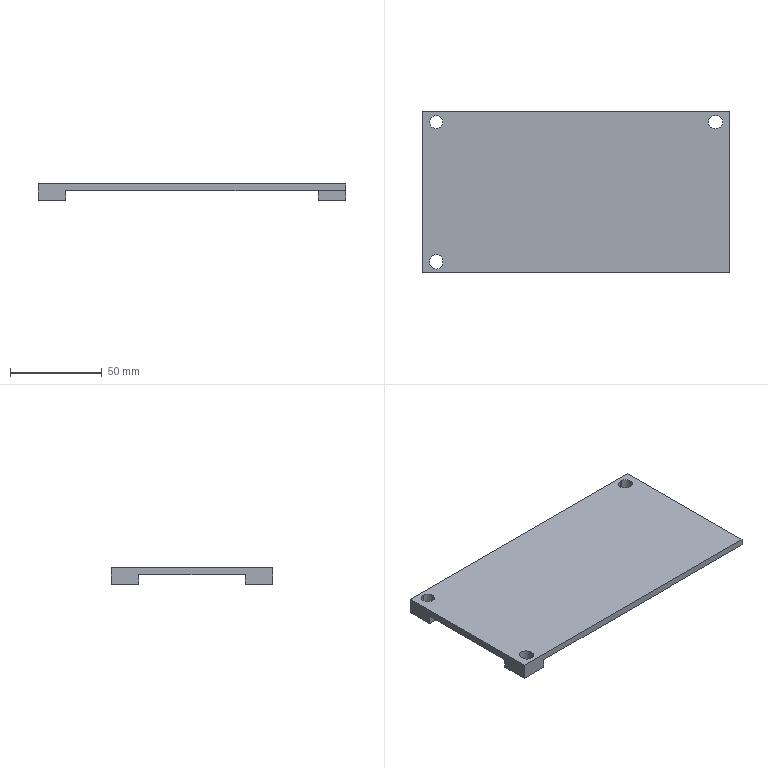NC program | NX | posted with a generic post | part box 168 x 88.2 x 8.8 mm
Lines 883 to 1702 of 6992:
(ZLEVEL_PROFILE , TOOL : D4)
N1752 T11 M6
N1754 G54
N1756 G17 G0 G90 X77.772 Y39.189 S9500 M3
N1758 G43 Z30. H11
N1760 Z1.5
N1762 G94 G1 X77.523 Y39.412 Z1.483 F1000.
N1764 X77.175 Y39.593 Z1.462
N1766 X76.793 Y39.685 Z1.441
N1768 X75.607 Z1.379
N1770 X75.225 Y39.594 Z1.359
N1772 X74.878 Y39.412 Z1.338
N1774 X74.585 Y39.151 Z1.318
N1776 X74.365 Y38.826 Z1.297
N1778 X74.239 Y38.492 Z1.278
N1780 X74.191 Y38.043 Z1.255
N1782 X74.271 Y37.597 Z1.231
N1784 X74.473 Y37.193 Z1.207
N1786 X74.781 Y36.861 Z1.183
N1788 X75.169 Y36.629 Z1.16
N1790 X75.607 Y36.515 Z1.136
N1792 X76.793 Z1.074
N1794 X77.231 Y36.629 Z1.05
N1796 X77.619 Y36.861 Z1.026
N1798 X77.927 Y37.192 Z1.003
N1800 X78.129 Y37.597 Z0.979
N1802 X78.209 Y38.042 Z0.955
N1804 X78.161 Y38.492 Z0.932
N1806 X78.036 Y38.825 Z0.913
N1808 X77.815 Y39.15 Z0.892
N1810 X77.523 Y39.412 Z0.872
N1812 X77.175 Y39.593 Z0.851
N1814 X76.793 Y39.685 Z0.831
N1816 X75.607 Z0.769
N1818 X75.225 Y39.594 Z0.748
N1820 X74.878 Y39.412 Z0.727
N1822 X74.585 Y39.151 Z0.707
N1824 X74.365 Y38.826 Z0.686
N1826 X74.239 Y38.492 Z0.668
N1828 X74.191 Y38.043 Z0.644
N1830 X74.271 Y37.597 Z0.62
N1832 X74.473 Y37.193 Z0.596
N1834 X74.781 Y36.861 Z0.573
N1836 X75.169 Y36.629 Z0.549
N1838 X75.607 Y36.515 Z0.525
N1840 X76.793 Z0.463
N1842 X77.231 Y36.629 Z0.439
N1844 X77.619 Y36.861 Z0.416
N1846 X77.927 Y37.192 Z0.392
N1848 X78.129 Y37.597 Z0.368
N1850 X78.209 Y38.042 Z0.345
N1852 X78.161 Y38.492 Z0.321
N1854 X78.036 Y38.825 Z0.302
N1856 X77.815 Y39.15 Z0.282
N1858 X77.523 Y39.412 Z0.261
N1860 X77.175 Y39.593 Z0.241
N1862 X76.793 Y39.685 Z0.22
N1864 X75.607 Z0.158
N1866 X75.225 Y39.594 Z0.137
N1868 X74.878 Y39.412 Z0.117
N1870 X74.585 Y39.151 Z0.096
N1872 X74.365 Y38.826 Z0.076
N1874 X74.239 Y38.492 Z0.057
N1876 X74.191 Y38.043 Z0.033
N1878 X74.271 Y37.597 Z0.01
N1880 X74.473 Y37.193 Z-0.014
N1882 X74.781 Y36.861 Z-0.038
N1884 X75.169 Y36.629 Z-0.062
N1886 X75.607 Y36.515 Z-0.085
N1888 X76.793 Z-0.148
N1890 X77.231 Y36.629 Z-0.171
N1892 X77.619 Y36.861 Z-0.195
N1894 X77.927 Y37.192 Z-0.219
N1896 X78.129 Y37.597 Z-0.242
N1898 X78.209 Y38.042 Z-0.266
N1900 X78.161 Y38.492 Z-0.29
N1902 X78.036 Y38.825 Z-0.308
N1904 X77.815 Y39.15 Z-0.329
N1906 X77.523 Y39.412 Z-0.35
N1908 X77.175 Y39.593 Z-0.37
N1910 X76.793 Y39.685 Z-0.391
N1912 X76.615 Z-0.4
N1914 X75.785 F2000.
N1916 G3 X74.2 Y38.1 R1.585
N1918 X75.785 Y36.515 R1.585
N1920 G1 X76.615
N1922 G3 X78.2 Y38.1 R1.585
N1924 X76.615 Y39.685 R1.585
N1926 G1 X75.785 Z-0.429
N1928 X75.625 Y39.677 Z-0.434
N1930 X75.467 Y39.653 Z-0.44
N1932 X75.349 Y39.624 Z-0.444
N1934 X75.248 Y39.591 Z-0.447
N1936 X75.163 Y39.558 Z-0.451
N1938 X75.046 Y39.502 Z-0.455
N1940 X74.953 Y39.449 Z-0.459
N1942 X74.883 Y39.404 Z-0.462
N1944 X74.779 Y39.325 Z-0.466
N1946 X74.699 Y39.255 Z-0.47
N1948 X74.64 Y39.196 Z-0.473
N1950 X74.554 Y39.098 Z-0.477
N1952 X74.49 Y39.014 Z-0.481
N1954 X74.444 Y38.945 Z-0.484
N1956 X74.378 Y38.83 Z-0.488
N1958 X74.332 Y38.734 Z-0.492
N1960 X74.302 Y38.659 Z-0.495
N1962 X74.258 Y38.526 Z-0.499
N1964 X74.232 Y38.416 Z-0.503
N1966 X74.217 Y38.33 Z-0.506
N1968 X74.203 Y38.192 Z-0.511
N1970 X74.2 Y38.079 Z-0.515
N1972 X74.204 Y37.991 Z-0.518
N1974 X74.219 Y37.853 Z-0.523
N1976 X74.241 Y37.742 Z-0.527
N1978 X74.263 Y37.657 Z-0.53
N1980 X74.308 Y37.525 Z-0.535
N1982 X74.353 Y37.421 Z-0.538
N1984 X74.392 Y37.343 Z-0.541
N1986 X74.464 Y37.224 Z-0.546
N1988 X74.53 Y37.132 Z-0.55
N1990 X74.586 Y37.064 Z-0.553
N1992 X74.681 Y36.963 Z-0.558
N1994 X74.765 Y36.887 Z-0.562
N1996 X74.834 Y36.832 Z-0.565
N1998 X74.949 Y36.754 Z-0.57
N2000 X75.047 Y36.697 Z-0.574
N2002 X75.125 Y36.659 Z-0.577
N2004 X75.254 Y36.606 Z-0.581
N2006 X75.362 Y36.572 Z-0.585
N2008 X75.447 Y36.551 Z-0.588
N2010 X75.615 Y36.524 Z-0.594
N2012 X75.785 Y36.515 Z-0.6
N2014 X76.615 Z-0.629
N2016 X76.766 Y36.522 Z-0.634
N2018 X76.878 Y36.537 Z-0.638
N2020 X76.952 Y36.551 Z-0.64
N2022 X77.088 Y36.587 Z-0.645
N2024 X77.195 Y36.625 Z-0.649
N2026 X77.274 Y36.659 Z-0.652
N2028 X77.398 Y36.722 Z-0.657
N2030 X77.495 Y36.782 Z-0.661
N2032 X77.566 Y36.832 Z-0.664
N2034 X77.674 Y36.92 Z-0.669
N2036 X77.755 Y36.999 Z-0.672
N2038 X77.814 Y37.064 Z-0.675
N2040 X77.901 Y37.173 Z-0.68
N2042 X77.963 Y37.267 Z-0.684
N2044 X78.007 Y37.343 Z-0.687
N2046 X78.068 Y37.468 Z-0.692
N2048 X78.11 Y37.573 Z-0.696
N2050 X78.137 Y37.657 Z-0.699
N2052 X78.17 Y37.792 Z-0.704
N2054 X78.188 Y37.903 Z-0.708
N2056 X78.196 Y37.991 Z-0.711
N2058 X78.2 Y38.13 Z-0.715
N2060 X78.194 Y38.243 Z-0.719
N2062 X78.183 Y38.33 Z-0.722
N2064 X78.157 Y38.465 Z-0.727
N2066 X78.127 Y38.574 Z-0.731
N2068 X78.098 Y38.658 Z-0.734
N2070 X78.048 Y38.778 Z-0.738
N2072 X77.999 Y38.873 Z-0.742
N2074 X77.956 Y38.944 Z-0.745
N2076 X77.882 Y39.052 Z-0.749
N2078 X77.815 Y39.135 Z-0.753
N2080 X77.76 Y39.196 Z-0.756
N2082 X77.666 Y39.287 Z-0.76
N2084 X77.584 Y39.355 Z-0.764
N2086 X77.517 Y39.403 Z-0.767
N2088 X77.406 Y39.473 Z-0.771
N2090 X77.312 Y39.523 Z-0.775
N2092 X77.237 Y39.558 Z-0.778
N2094 X77.115 Y39.604 Z-0.782
N2096 X77.013 Y39.634 Z-0.786
N2098 X76.933 Y39.653 Z-0.789
N2100 X76.775 Y39.677 Z-0.794
N2102 X76.615 Y39.685 Z-0.8
N2104 X75.785 Z-0.829
N2106 X75.625 Y39.677 Z-0.834
N2108 X75.467 Y39.653 Z-0.84
N2110 X75.349 Y39.624 Z-0.844
N2112 X75.248 Y39.591 Z-0.847
N2114 X75.163 Y39.558 Z-0.851
N2116 X75.046 Y39.502 Z-0.855
N2118 X74.953 Y39.449 Z-0.859
N2120 X74.883 Y39.404 Z-0.862
N2122 X74.779 Y39.325 Z-0.866
N2124 X74.699 Y39.255 Z-0.87
N2126 X74.64 Y39.196 Z-0.873
N2128 X74.554 Y39.098 Z-0.877
N2130 X74.49 Y39.014 Z-0.881
N2132 X74.444 Y38.945 Z-0.884
N2134 X74.378 Y38.83 Z-0.888
N2136 X74.332 Y38.734 Z-0.892
N2138 X74.302 Y38.659 Z-0.895
N2140 X74.258 Y38.526 Z-0.899
N2142 X74.232 Y38.416 Z-0.903
N2144 X74.217 Y38.33 Z-0.906
N2146 X74.203 Y38.192 Z-0.911
N2148 X74.2 Y38.079 Z-0.915
N2150 X74.204 Y37.991 Z-0.918
N2152 X74.219 Y37.853 Z-0.923
N2154 X74.241 Y37.742 Z-0.927
N2156 X74.263 Y37.657 Z-0.93
N2158 X74.308 Y37.525 Z-0.935
N2160 X74.353 Y37.421 Z-0.938
N2162 X74.392 Y37.343 Z-0.941
N2164 X74.464 Y37.224 Z-0.946
N2166 X74.53 Y37.132 Z-0.95
N2168 X74.586 Y37.064 Z-0.953
N2170 X74.681 Y36.963 Z-0.958
N2172 X74.765 Y36.887 Z-0.962
N2174 X74.834 Y36.832 Z-0.965
N2176 X74.949 Y36.754 Z-0.97
N2178 X75.047 Y36.697 Z-0.974
N2180 X75.125 Y36.659 Z-0.977
N2182 X75.254 Y36.606 Z-0.981
N2184 X75.362 Y36.572 Z-0.985
N2186 X75.447 Y36.551 Z-0.988
N2188 X75.615 Y36.524 Z-0.994
N2190 X75.785 Y36.515 Z-1.
N2192 X76.615 Z-1.029
N2194 X76.766 Y36.522 Z-1.034
N2196 X76.878 Y36.537 Z-1.038
N2198 X76.952 Y36.551 Z-1.04
N2200 X77.088 Y36.587 Z-1.045
N2202 X77.195 Y36.625 Z-1.049
N2204 X77.274 Y36.659 Z-1.052
N2206 X77.398 Y36.722 Z-1.057
N2208 X77.495 Y36.782 Z-1.061
N2210 X77.566 Y36.832 Z-1.064
N2212 X77.674 Y36.92 Z-1.069
N2214 X77.755 Y36.999 Z-1.072
N2216 X77.814 Y37.064 Z-1.075
N2218 X77.901 Y37.173 Z-1.08
N2220 X77.963 Y37.267 Z-1.084
N2222 X78.007 Y37.343 Z-1.087
N2224 X78.068 Y37.468 Z-1.092
N2226 X78.11 Y37.573 Z-1.096
N2228 X78.137 Y37.657 Z-1.099
N2230 X78.17 Y37.792 Z-1.104
N2232 X78.188 Y37.903 Z-1.108
N2234 X78.196 Y37.991 Z-1.111
N2236 X78.2 Y38.13 Z-1.115
N2238 X78.194 Y38.243 Z-1.119
N2240 X78.183 Y38.33 Z-1.122
N2242 X78.157 Y38.465 Z-1.127
N2244 X78.127 Y38.574 Z-1.131
N2246 X78.098 Y38.658 Z-1.134
N2248 X78.048 Y38.778 Z-1.138
N2250 X77.999 Y38.873 Z-1.142
N2252 X77.956 Y38.944 Z-1.145
N2254 X77.882 Y39.052 Z-1.149
N2256 X77.815 Y39.135 Z-1.153
N2258 X77.76 Y39.196 Z-1.156
N2260 X77.666 Y39.287 Z-1.16
N2262 X77.584 Y39.355 Z-1.164
N2264 X77.517 Y39.403 Z-1.167
N2266 X77.406 Y39.473 Z-1.171
N2268 X77.312 Y39.523 Z-1.175
N2270 X77.237 Y39.558 Z-1.178
N2272 X77.115 Y39.604 Z-1.182
N2274 X77.013 Y39.634 Z-1.186
N2276 X76.933 Y39.653 Z-1.189
N2278 X76.775 Y39.677 Z-1.194
N2280 X76.615 Y39.685 Z-1.2
N2282 X75.785 Z-1.229
N2284 X75.625 Y39.677 Z-1.234
N2286 X75.467 Y39.653 Z-1.24
N2288 X75.349 Y39.624 Z-1.244
N2290 X75.248 Y39.591 Z-1.247
N2292 X75.163 Y39.558 Z-1.251
N2294 X75.046 Y39.502 Z-1.255
N2296 X74.953 Y39.449 Z-1.259
N2298 X74.883 Y39.404 Z-1.262
N2300 X74.779 Y39.325 Z-1.266
N2302 X74.699 Y39.255 Z-1.27
N2304 X74.64 Y39.196 Z-1.273
N2306 X74.554 Y39.098 Z-1.277
N2308 X74.49 Y39.014 Z-1.281
N2310 X74.444 Y38.945 Z-1.284
N2312 X74.378 Y38.83 Z-1.288
N2314 X74.332 Y38.734 Z-1.292
N2316 X74.302 Y38.659 Z-1.295
N2318 X74.258 Y38.526 Z-1.299
N2320 X74.232 Y38.416 Z-1.303
N2322 X74.217 Y38.33 Z-1.306
N2324 X74.203 Y38.192 Z-1.311
N2326 X74.2 Y38.079 Z-1.315
N2328 X74.204 Y37.991 Z-1.318
N2330 X74.219 Y37.853 Z-1.323
N2332 X74.241 Y37.742 Z-1.327
N2334 X74.263 Y37.657 Z-1.33
N2336 X74.308 Y37.525 Z-1.335
N2338 X74.353 Y37.421 Z-1.338
N2340 X74.392 Y37.343 Z-1.341
N2342 X74.464 Y37.224 Z-1.346
N2344 X74.53 Y37.132 Z-1.35
N2346 X74.586 Y37.064 Z-1.353
N2348 X74.681 Y36.963 Z-1.358
N2350 X74.765 Y36.887 Z-1.362
N2352 X74.834 Y36.832 Z-1.365
N2354 X74.949 Y36.754 Z-1.37
N2356 X75.047 Y36.697 Z-1.374
N2358 X75.125 Y36.659 Z-1.377
N2360 X75.254 Y36.606 Z-1.381
N2362 X75.362 Y36.572 Z-1.385
N2364 X75.447 Y36.551 Z-1.388
N2366 X75.615 Y36.524 Z-1.394
N2368 X75.785 Y36.515 Z-1.4
N2370 X76.615 Z-1.429
N2372 X76.766 Y36.522 Z-1.434
N2374 X76.878 Y36.537 Z-1.438
N2376 X76.952 Y36.551 Z-1.44
N2378 X77.088 Y36.587 Z-1.445
N2380 X77.195 Y36.625 Z-1.449
N2382 X77.274 Y36.659 Z-1.452
N2384 X77.398 Y36.722 Z-1.457
N2386 X77.495 Y36.782 Z-1.461
N2388 X77.566 Y36.832 Z-1.464
N2390 X77.674 Y36.92 Z-1.469
N2392 X77.755 Y36.999 Z-1.472
N2394 X77.814 Y37.064 Z-1.475
N2396 X77.901 Y37.173 Z-1.48
N2398 X77.963 Y37.267 Z-1.484
N2400 X78.007 Y37.343 Z-1.487
N2402 X78.068 Y37.468 Z-1.492
N2404 X78.11 Y37.573 Z-1.496
N2406 X78.137 Y37.657 Z-1.499
N2408 X78.17 Y37.792 Z-1.504
N2410 X78.188 Y37.903 Z-1.508
N2412 X78.196 Y37.991 Z-1.511
N2414 X78.2 Y38.13 Z-1.515
N2416 X78.194 Y38.243 Z-1.519
N2418 X78.183 Y38.33 Z-1.522
N2420 X78.157 Y38.465 Z-1.527
N2422 X78.127 Y38.574 Z-1.531
N2424 X78.098 Y38.658 Z-1.534
N2426 X78.048 Y38.778 Z-1.538
N2428 X77.999 Y38.873 Z-1.542
N2430 X77.956 Y38.944 Z-1.545
N2432 X77.882 Y39.052 Z-1.549
N2434 X77.815 Y39.135 Z-1.553
N2436 X77.76 Y39.196 Z-1.556
N2438 X77.666 Y39.287 Z-1.56
N2440 X77.584 Y39.355 Z-1.564
N2442 X77.517 Y39.403 Z-1.567
N2444 X77.406 Y39.473 Z-1.571
N2446 X77.312 Y39.523 Z-1.575
N2448 X77.237 Y39.558 Z-1.578
N2450 X77.115 Y39.604 Z-1.582
N2452 X77.013 Y39.634 Z-1.586
N2454 X76.933 Y39.653 Z-1.589
N2456 X76.775 Y39.677 Z-1.594
N2458 X76.615 Y39.685 Z-1.6
N2460 X75.785 Z-1.629
N2462 X75.625 Y39.677 Z-1.634
N2464 X75.467 Y39.653 Z-1.64
N2466 X75.349 Y39.624 Z-1.644
N2468 X75.248 Y39.591 Z-1.647
N2470 X75.163 Y39.558 Z-1.651
N2472 X75.046 Y39.502 Z-1.655
N2474 X74.953 Y39.449 Z-1.659
N2476 X74.883 Y39.404 Z-1.662
N2478 X74.779 Y39.325 Z-1.666
N2480 X74.699 Y39.255 Z-1.67
N2482 X74.64 Y39.196 Z-1.673
N2484 X74.554 Y39.098 Z-1.677
N2486 X74.49 Y39.014 Z-1.681
N2488 X74.444 Y38.945 Z-1.684
N2490 X74.378 Y38.83 Z-1.688
N2492 X74.332 Y38.734 Z-1.692
N2494 X74.302 Y38.659 Z-1.695
N2496 X74.258 Y38.526 Z-1.699
N2498 X74.232 Y38.416 Z-1.703
N2500 X74.217 Y38.33 Z-1.706
N2502 X74.203 Y38.192 Z-1.711
N2504 X74.2 Y38.079 Z-1.715
N2506 X74.204 Y37.991 Z-1.718
N2508 X74.219 Y37.853 Z-1.723
N2510 X74.241 Y37.742 Z-1.727
N2512 X74.263 Y37.657 Z-1.73
N2514 X74.308 Y37.525 Z-1.735
N2516 X74.353 Y37.421 Z-1.738
N2518 X74.392 Y37.343 Z-1.741
N2520 X74.464 Y37.224 Z-1.746
N2522 X74.53 Y37.132 Z-1.75
N2524 X74.586 Y37.064 Z-1.753
N2526 X74.681 Y36.963 Z-1.758
N2528 X74.765 Y36.887 Z-1.762
N2530 X74.834 Y36.832 Z-1.765
N2532 X74.949 Y36.754 Z-1.77
N2534 X75.047 Y36.697 Z-1.774
N2536 X75.125 Y36.659 Z-1.777
N2538 X75.254 Y36.606 Z-1.781
N2540 X75.362 Y36.572 Z-1.785
N2542 X75.447 Y36.551 Z-1.788
N2544 X75.615 Y36.524 Z-1.794
N2546 X75.785 Y36.515 Z-1.8
N2548 X76.615 Z-1.829
N2550 X76.766 Y36.522 Z-1.834
N2552 X76.878 Y36.537 Z-1.838
N2554 X76.952 Y36.551 Z-1.84
N2556 X77.088 Y36.587 Z-1.845
N2558 X77.195 Y36.625 Z-1.849
N2560 X77.274 Y36.659 Z-1.852
N2562 X77.398 Y36.722 Z-1.857
N2564 X77.495 Y36.782 Z-1.861
N2566 X77.566 Y36.832 Z-1.864
N2568 X77.674 Y36.92 Z-1.869
N2570 X77.755 Y36.999 Z-1.872
N2572 X77.814 Y37.064 Z-1.875
N2574 X77.901 Y37.173 Z-1.88
N2576 X77.963 Y37.267 Z-1.884
N2578 X78.007 Y37.343 Z-1.887
N2580 X78.068 Y37.468 Z-1.892
N2582 X78.11 Y37.573 Z-1.896
N2584 X78.137 Y37.657 Z-1.899
N2586 X78.17 Y37.792 Z-1.904
N2588 X78.188 Y37.903 Z-1.908
N2590 X78.196 Y37.991 Z-1.911
N2592 X78.2 Y38.13 Z-1.915
N2594 X78.194 Y38.243 Z-1.919
N2596 X78.183 Y38.33 Z-1.922
N2598 X78.157 Y38.465 Z-1.927
N2600 X78.127 Y38.574 Z-1.931
N2602 X78.098 Y38.658 Z-1.934
N2604 X78.048 Y38.778 Z-1.938
N2606 X77.999 Y38.873 Z-1.942
N2608 X77.956 Y38.944 Z-1.945
N2610 X77.882 Y39.052 Z-1.949
N2612 X77.815 Y39.135 Z-1.953
N2614 X77.76 Y39.196 Z-1.956
N2616 X77.666 Y39.287 Z-1.96
N2618 X77.584 Y39.355 Z-1.964
N2620 X77.517 Y39.403 Z-1.967
N2622 X77.406 Y39.473 Z-1.971
N2624 X77.312 Y39.523 Z-1.975
N2626 X77.237 Y39.558 Z-1.978
N2628 X77.115 Y39.604 Z-1.982
N2630 X77.013 Y39.634 Z-1.986
N2632 X76.933 Y39.653 Z-1.989
N2634 X76.775 Y39.677 Z-1.994
N2636 X76.615 Y39.685 Z-2.
N2638 X75.785 Z-2.029
N2640 X75.625 Y39.677 Z-2.034
N2642 X75.467 Y39.653 Z-2.04
N2644 X75.349 Y39.624 Z-2.044
N2646 X75.248 Y39.591 Z-2.047
N2648 X75.163 Y39.558 Z-2.051
N2650 X75.046 Y39.502 Z-2.055
N2652 X74.953 Y39.449 Z-2.059
N2654 X74.883 Y39.404 Z-2.062
N2656 X74.779 Y39.325 Z-2.066
N2658 X74.699 Y39.255 Z-2.07
N2660 X74.64 Y39.196 Z-2.073
N2662 X74.554 Y39.098 Z-2.077
N2664 X74.49 Y39.014 Z-2.081
N2666 X74.444 Y38.945 Z-2.084
N2668 X74.378 Y38.83 Z-2.088
N2670 X74.332 Y38.734 Z-2.092
N2672 X74.302 Y38.659 Z-2.095
N2674 X74.258 Y38.526 Z-2.099
N2676 X74.232 Y38.416 Z-2.103
N2678 X74.217 Y38.33 Z-2.106
N2680 X74.203 Y38.192 Z-2.111
N2682 X74.2 Y38.079 Z-2.115
N2684 X74.204 Y37.991 Z-2.118
N2686 X74.219 Y37.853 Z-2.123
N2688 X74.241 Y37.742 Z-2.127
N2690 X74.263 Y37.657 Z-2.13
N2692 X74.308 Y37.525 Z-2.135
N2694 X74.353 Y37.421 Z-2.138
N2696 X74.392 Y37.343 Z-2.141
N2698 X74.464 Y37.224 Z-2.146
N2700 X74.53 Y37.132 Z-2.15
N2702 X74.586 Y37.064 Z-2.153
N2704 X74.681 Y36.963 Z-2.158
N2706 X74.765 Y36.887 Z-2.162
N2708 X74.834 Y36.832 Z-2.165
N2710 X74.949 Y36.754 Z-2.17
N2712 X75.047 Y36.697 Z-2.174
N2714 X75.125 Y36.659 Z-2.177
N2716 X75.254 Y36.606 Z-2.181
N2718 X75.362 Y36.572 Z-2.185
N2720 X75.447 Y36.551 Z-2.188
N2722 X75.615 Y36.524 Z-2.194
N2724 X75.785 Y36.515 Z-2.2
N2726 X76.615 Z-2.229
N2728 X76.766 Y36.522 Z-2.234
N2730 X76.878 Y36.537 Z-2.238
N2732 X76.952 Y36.551 Z-2.24
N2734 X77.088 Y36.587 Z-2.245
N2736 X77.195 Y36.625 Z-2.249
N2738 X77.274 Y36.659 Z-2.252
N2740 X77.398 Y36.722 Z-2.257
N2742 X77.495 Y36.782 Z-2.261
N2744 X77.566 Y36.832 Z-2.264
N2746 X77.674 Y36.92 Z-2.269
N2748 X77.755 Y36.999 Z-2.272
N2750 X77.814 Y37.064 Z-2.275
N2752 X77.901 Y37.173 Z-2.28
N2754 X77.963 Y37.267 Z-2.284
N2756 X78.007 Y37.343 Z-2.287
N2758 X78.068 Y37.468 Z-2.292
N2760 X78.11 Y37.573 Z-2.296
N2762 X78.137 Y37.657 Z-2.299
N2764 X78.17 Y37.792 Z-2.304
N2766 X78.188 Y37.903 Z-2.308
N2768 X78.196 Y37.991 Z-2.311
N2770 X78.2 Y38.13 Z-2.315
N2772 X78.194 Y38.243 Z-2.319
N2774 X78.183 Y38.33 Z-2.322
N2776 X78.157 Y38.465 Z-2.327
N2778 X78.127 Y38.574 Z-2.331
N2780 X78.098 Y38.658 Z-2.334
N2782 X78.048 Y38.778 Z-2.338
N2784 X77.999 Y38.873 Z-2.342
N2786 X77.956 Y38.944 Z-2.345
N2788 X77.882 Y39.052 Z-2.349
N2790 X77.815 Y39.135 Z-2.353
N2792 X77.76 Y39.196 Z-2.356
N2794 X77.666 Y39.287 Z-2.36
N2796 X77.584 Y39.355 Z-2.364
N2798 X77.517 Y39.403 Z-2.367
N2800 X77.406 Y39.473 Z-2.371
N2802 X77.312 Y39.523 Z-2.375
N2804 X77.237 Y39.558 Z-2.378
N2806 X77.115 Y39.604 Z-2.382
N2808 X77.013 Y39.634 Z-2.386
N2810 X76.933 Y39.653 Z-2.389
N2812 X76.775 Y39.677 Z-2.394
N2814 X76.615 Y39.685 Z-2.4
N2816 X75.785 Z-2.429
N2818 X75.625 Y39.677 Z-2.434
N2820 X75.467 Y39.653 Z-2.44
N2822 X75.349 Y39.624 Z-2.444
N2824 X75.248 Y39.591 Z-2.447
N2826 X75.163 Y39.558 Z-2.451
N2828 X75.046 Y39.502 Z-2.455
N2830 X74.953 Y39.449 Z-2.459
N2832 X74.883 Y39.404 Z-2.462
N2834 X74.779 Y39.325 Z-2.466
N2836 X74.699 Y39.255 Z-2.47
N2838 X74.64 Y39.196 Z-2.473
N2840 X74.554 Y39.098 Z-2.477
N2842 X74.49 Y39.014 Z-2.481
N2844 X74.444 Y38.945 Z-2.484
N2846 X74.378 Y38.83 Z-2.488
N2848 X74.332 Y38.734 Z-2.492
N2850 X74.302 Y38.659 Z-2.495
N2852 X74.258 Y38.526 Z-2.499
N2854 X74.232 Y38.416 Z-2.503
N2856 X74.217 Y38.33 Z-2.506
N2858 X74.203 Y38.192 Z-2.511
N2860 X74.2 Y38.079 Z-2.515
N2862 X74.204 Y37.991 Z-2.518
N2864 X74.219 Y37.853 Z-2.523
N2866 X74.241 Y37.742 Z-2.527
N2868 X74.263 Y37.657 Z-2.53
N2870 X74.308 Y37.525 Z-2.535
N2872 X74.353 Y37.421 Z-2.538
N2874 X74.392 Y37.343 Z-2.541
N2876 X74.464 Y37.224 Z-2.546
N2878 X74.53 Y37.132 Z-2.55
N2880 X74.586 Y37.064 Z-2.553
N2882 X74.681 Y36.963 Z-2.558
N2884 X74.765 Y36.887 Z-2.562
N2886 X74.834 Y36.832 Z-2.565
N2888 X74.949 Y36.754 Z-2.57
N2890 X75.047 Y36.697 Z-2.574
N2892 X75.125 Y36.659 Z-2.577
N2894 X75.254 Y36.606 Z-2.581
N2896 X75.362 Y36.572 Z-2.585
N2898 X75.447 Y36.551 Z-2.588
N2900 X75.615 Y36.524 Z-2.594
N2902 X75.785 Y36.515 Z-2.6
N2904 X76.615 Z-2.629
N2906 X76.766 Y36.522 Z-2.634
N2908 X76.878 Y36.537 Z-2.638
N2910 X76.952 Y36.551 Z-2.64
N2912 X77.088 Y36.587 Z-2.645
N2914 X77.195 Y36.625 Z-2.649
N2916 X77.274 Y36.659 Z-2.652
N2918 X77.398 Y36.722 Z-2.657
N2920 X77.495 Y36.782 Z-2.661
N2922 X77.566 Y36.832 Z-2.664
N2924 X77.674 Y36.92 Z-2.669
N2926 X77.755 Y36.999 Z-2.672
N2928 X77.814 Y37.064 Z-2.675
N2930 X77.901 Y37.173 Z-2.68
N2932 X77.963 Y37.267 Z-2.684
N2934 X78.007 Y37.343 Z-2.687
N2936 X78.068 Y37.468 Z-2.692
N2938 X78.11 Y37.573 Z-2.696
N2940 X78.137 Y37.657 Z-2.699
N2942 X78.17 Y37.792 Z-2.704
N2944 X78.188 Y37.903 Z-2.708
N2946 X78.196 Y37.991 Z-2.711
N2948 X78.2 Y38.13 Z-2.715
N2950 X78.194 Y38.243 Z-2.719
N2952 X78.183 Y38.33 Z-2.722
N2954 X78.157 Y38.465 Z-2.727
N2956 X78.127 Y38.574 Z-2.731
N2958 X78.098 Y38.658 Z-2.734
N2960 X78.048 Y38.778 Z-2.738
N2962 X77.999 Y38.873 Z-2.742
N2964 X77.956 Y38.944 Z-2.745
N2966 X77.882 Y39.052 Z-2.749
N2968 X77.815 Y39.135 Z-2.753
N2970 X77.76 Y39.196 Z-2.756
N2972 X77.666 Y39.287 Z-2.76
N2974 X77.584 Y39.355 Z-2.764
N2976 X77.517 Y39.403 Z-2.767
N2978 X77.406 Y39.473 Z-2.771
N2980 X77.312 Y39.523 Z-2.775
N2982 X77.237 Y39.558 Z-2.778
N2984 X77.115 Y39.604 Z-2.782
N2986 X77.013 Y39.634 Z-2.786
N2988 X76.933 Y39.653 Z-2.789
N2990 X76.775 Y39.677 Z-2.794
N2992 X76.615 Y39.685 Z-2.8
N2994 X75.785 Z-2.829
N2996 X75.625 Y39.677 Z-2.834
N2998 X75.467 Y39.653 Z-2.84
N3000 X75.349 Y39.624 Z-2.844
N3002 X75.248 Y39.591 Z-2.847
N3004 X75.163 Y39.558 Z-2.851
N3006 X75.046 Y39.502 Z-2.855
N3008 X74.953 Y39.449 Z-2.859
N3010 X74.883 Y39.404 Z-2.862
N3012 X74.779 Y39.325 Z-2.866
N3014 X74.699 Y39.255 Z-2.87
N3016 X74.64 Y39.196 Z-2.873
N3018 X74.554 Y39.098 Z-2.877
N3020 X74.49 Y39.014 Z-2.881
N3022 X74.444 Y38.945 Z-2.884
N3024 X74.378 Y38.83 Z-2.888
N3026 X74.332 Y38.734 Z-2.892
N3028 X74.302 Y38.659 Z-2.895
N3030 X74.258 Y38.526 Z-2.899
N3032 X74.232 Y38.416 Z-2.903
N3034 X74.217 Y38.33 Z-2.906
N3036 X74.203 Y38.192 Z-2.911
N3038 X74.2 Y38.079 Z-2.915
N3040 X74.204 Y37.991 Z-2.918
N3042 X74.219 Y37.853 Z-2.923
N3044 X74.241 Y37.742 Z-2.927
N3046 X74.263 Y37.657 Z-2.93
N3048 X74.308 Y37.525 Z-2.935
N3050 X74.353 Y37.421 Z-2.938
N3052 X74.392 Y37.343 Z-2.941
N3054 X74.464 Y37.224 Z-2.946
N3056 X74.53 Y37.132 Z-2.95
N3058 X74.586 Y37.064 Z-2.953
N3060 X74.681 Y36.963 Z-2.958
N3062 X74.765 Y36.887 Z-2.962
N3064 X74.834 Y36.832 Z-2.965
N3066 X74.949 Y36.754 Z-2.97
N3068 X75.047 Y36.697 Z-2.974
N3070 X75.125 Y36.659 Z-2.977
N3072 X75.254 Y36.606 Z-2.981
N3074 X75.362 Y36.572 Z-2.985
N3076 X75.447 Y36.551 Z-2.988
N3078 X75.615 Y36.524 Z-2.994
N3080 X75.785 Y36.515 Z-3.
N3082 X76.615 Z-3.029
N3084 X76.766 Y36.522 Z-3.034
N3086 X76.878 Y36.537 Z-3.038
N3088 X76.952 Y36.551 Z-3.04
N3090 X77.088 Y36.587 Z-3.045
N3092 X77.195 Y36.625 Z-3.049
N3094 X77.274 Y36.659 Z-3.052
N3096 X77.398 Y36.722 Z-3.057
N3098 X77.495 Y36.782 Z-3.061
N3100 X77.566 Y36.832 Z-3.064
N3102 X77.674 Y36.92 Z-3.069
N3104 X77.755 Y36.999 Z-3.072
N3106 X77.814 Y37.064 Z-3.075
N3108 X77.901 Y37.173 Z-3.08
N3110 X77.963 Y37.267 Z-3.084
N3112 X78.007 Y37.343 Z-3.087
N3114 X78.068 Y37.468 Z-3.092
N3116 X78.11 Y37.573 Z-3.096
N3118 X78.137 Y37.657 Z-3.099
N3120 X78.17 Y37.792 Z-3.104
N3122 X78.188 Y37.903 Z-3.108
N3124 X78.196 Y37.991 Z-3.111
N3126 X78.2 Y38.13 Z-3.115
N3128 X78.194 Y38.243 Z-3.119
N3130 X78.183 Y38.33 Z-3.122
N3132 X78.157 Y38.465 Z-3.127
N3134 X78.127 Y38.574 Z-3.131
N3136 X78.098 Y38.658 Z-3.134
N3138 X78.048 Y38.778 Z-3.138
N3140 X77.999 Y38.873 Z-3.142
N3142 X77.956 Y38.944 Z-3.145
N3144 X77.882 Y39.052 Z-3.149
N3146 X77.815 Y39.135 Z-3.153
N3148 X77.76 Y39.196 Z-3.156
N3150 X77.666 Y39.287 Z-3.16
N3152 X77.584 Y39.355 Z-3.164
N3154 X77.517 Y39.403 Z-3.167
N3156 X77.406 Y39.473 Z-3.171
N3158 X77.312 Y39.523 Z-3.175
N3160 X77.237 Y39.558 Z-3.178
N3162 X77.115 Y39.604 Z-3.182
N3164 X77.013 Y39.634 Z-3.186
N3166 X76.933 Y39.653 Z-3.189
N3168 X76.775 Y39.677 Z-3.194
N3170 X76.615 Y39.685 Z-3.2
N3172 X75.785 Z-3.229
N3174 X75.625 Y39.677 Z-3.234
N3176 X75.467 Y39.653 Z-3.24
N3178 X75.349 Y39.624 Z-3.244
N3180 X75.248 Y39.591 Z-3.247
N3182 X75.163 Y39.558 Z-3.251
N3184 X75.046 Y39.502 Z-3.255
N3186 X74.953 Y39.449 Z-3.259
N3188 X74.883 Y39.404 Z-3.262
N3190 X74.779 Y39.325 Z-3.266
N3192 X74.699 Y39.255 Z-3.27
N3194 X74.64 Y39.196 Z-3.273
N3196 X74.554 Y39.098 Z-3.277
N3198 X74.49 Y39.014 Z-3.281
N3200 X74.444 Y38.945 Z-3.284
N3202 X74.378 Y38.83 Z-3.288
N3204 X74.332 Y38.734 Z-3.292
N3206 X74.302 Y38.659 Z-3.295
N3208 X74.258 Y38.526 Z-3.299
N3210 X74.232 Y38.416 Z-3.303
N3212 X74.217 Y38.33 Z-3.306
N3214 X74.203 Y38.192 Z-3.311
N3216 X74.2 Y38.079 Z-3.315
N3218 X74.204 Y37.991 Z-3.318
N3220 X74.219 Y37.853 Z-3.323
N3222 X74.241 Y37.742 Z-3.327
N3224 X74.263 Y37.657 Z-3.33
N3226 X74.308 Y37.525 Z-3.335
N3228 X74.353 Y37.421 Z-3.338
N3230 X74.392 Y37.343 Z-3.341
N3232 X74.464 Y37.224 Z-3.346
N3234 X74.53 Y37.132 Z-3.35
N3236 X74.586 Y37.064 Z-3.353
N3238 X74.681 Y36.963 Z-3.358
N3240 X74.765 Y36.887 Z-3.362
N3242 X74.834 Y36.832 Z-3.365
N3244 X74.949 Y36.754 Z-3.37
N3246 X75.047 Y36.697 Z-3.374
N3248 X75.125 Y36.659 Z-3.377
N3250 X75.254 Y36.606 Z-3.381
N3252 X75.362 Y36.572 Z-3.385
N3254 X75.447 Y36.551 Z-3.388
N3256 X75.615 Y36.524 Z-3.394
N3258 X75.785 Y36.515 Z-3.4
N3260 X76.615 Z-3.429
N3262 X76.766 Y36.522 Z-3.434
N3264 X76.878 Y36.537 Z-3.438
N3266 X76.952 Y36.551 Z-3.44
N3268 X77.088 Y36.587 Z-3.445
N3270 X77.195 Y36.625 Z-3.449
N3272 X77.274 Y36.659 Z-3.452
N3274 X77.398 Y36.722 Z-3.457
N3276 X77.495 Y36.782 Z-3.461
N3278 X77.566 Y36.832 Z-3.464
N3280 X77.674 Y36.92 Z-3.469
N3282 X77.755 Y36.999 Z-3.472
N3284 X77.814 Y37.064 Z-3.475
N3286 X77.901 Y37.173 Z-3.48
N3288 X77.963 Y37.267 Z-3.484
N3290 X78.007 Y37.343 Z-3.487
N3292 X78.068 Y37.468 Z-3.492
N3294 X78.11 Y37.573 Z-3.496
N3296 X78.137 Y37.657 Z-3.499
N3298 X78.17 Y37.792 Z-3.504
N3300 X78.188 Y37.903 Z-3.508
N3302 X78.196 Y37.991 Z-3.511
N3304 X78.2 Y38.13 Z-3.515
N3306 X78.194 Y38.243 Z-3.519
N3308 X78.183 Y38.33 Z-3.522
N3310 X78.157 Y38.465 Z-3.527
N3312 X78.127 Y38.574 Z-3.531
N3314 X78.098 Y38.658 Z-3.534
N3316 X78.048 Y38.778 Z-3.538
N3318 X77.999 Y38.873 Z-3.542
N3320 X77.956 Y38.944 Z-3.545
N3322 X77.882 Y39.052 Z-3.549
N3324 X77.815 Y39.135 Z-3.553
N3326 X77.76 Y39.196 Z-3.556
N3328 X77.666 Y39.287 Z-3.56
N3330 X77.584 Y39.355 Z-3.564
N3332 X77.517 Y39.403 Z-3.567
N3334 X77.406 Y39.473 Z-3.571
N3336 X77.312 Y39.523 Z-3.575
N3338 X77.237 Y39.558 Z-3.578
N3340 X77.115 Y39.604 Z-3.582
N3342 X77.013 Y39.634 Z-3.586
N3344 X76.933 Y39.653 Z-3.589
N3346 X76.775 Y39.677 Z-3.594
N3348 X76.615 Y39.685 Z-3.6
N3350 X75.785 Z-3.629
N3352 X75.625 Y39.677 Z-3.634
N3354 X75.467 Y39.653 Z-3.64
N3356 X75.349 Y39.624 Z-3.644
N3358 X75.248 Y39.591 Z-3.647
N3360 X75.163 Y39.558 Z-3.651
N3362 X75.046 Y39.502 Z-3.655
N3364 X74.953 Y39.449 Z-3.659
N3366 X74.883 Y39.404 Z-3.662
N3368 X74.779 Y39.325 Z-3.666
N3370 X74.699 Y39.255 Z-3.67
N3372 X74.64 Y39.196 Z-3.673
N3374 X74.554 Y39.098 Z-3.677
N3376 X74.49 Y39.014 Z-3.681
N3378 X74.444 Y38.945 Z-3.684
N3380 X74.378 Y38.83 Z-3.688
N3382 X74.332 Y38.734 Z-3.692
N3384 X74.302 Y38.659 Z-3.695